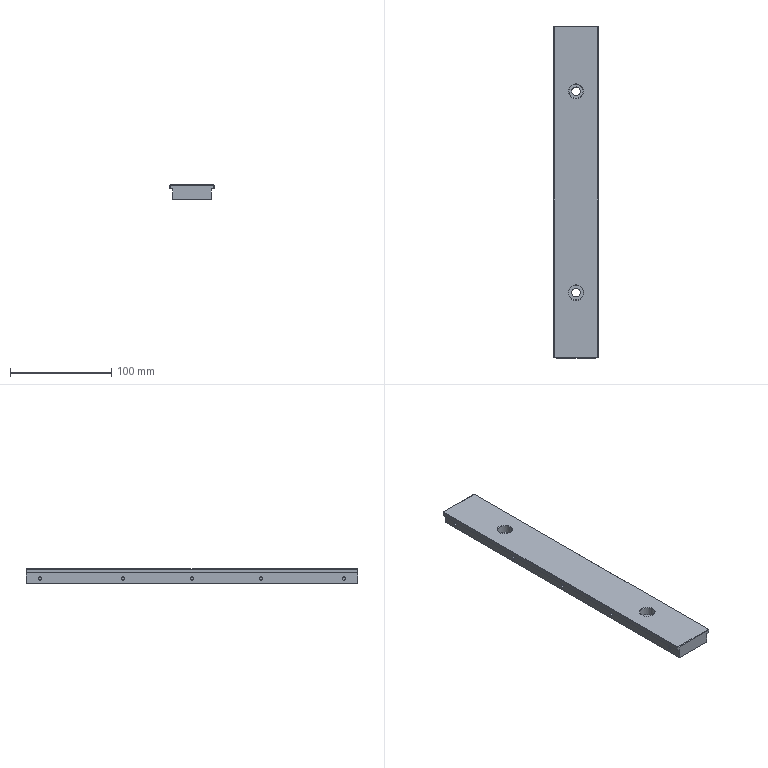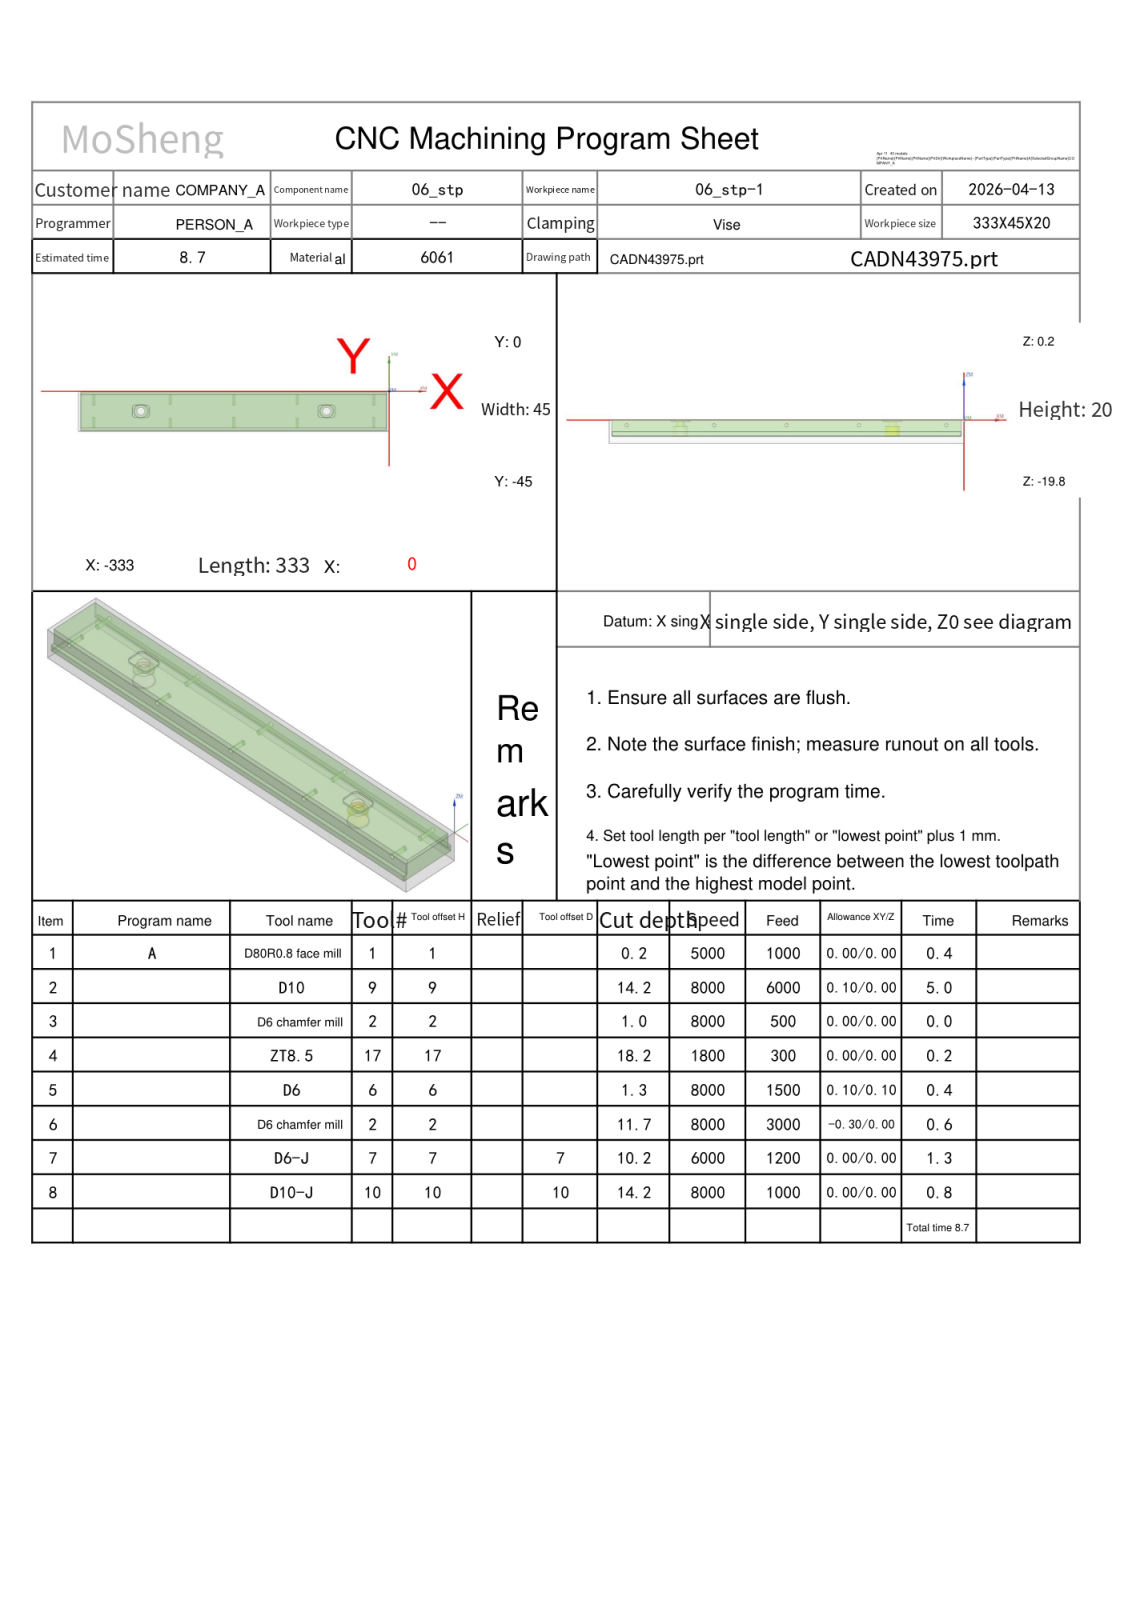NC program | NX | posted by the shop | part box 44 x 328 x 14 mm
Whole program:
%
O0001
(Machine time: 10.41 MIN)
(===Total Tool:7===)
(T1=D80R0.8 face mill D=80.  R=0.8  D-  H01 Z=-0.   )
(T9=D10     D=10.  R=0.   D-  H09 Z=-14.  )
(T2=D6 chamfer mill   D=6.   R=0.   D-  H02 Z=-11.5 )
(T17=ZT8.5  D=8.5  DR_a=118 D-  H17 Z=-18.  )
(T6=D6      D=6.   R=0.   D-  H06 Z=-1.1  )
(T7=D6-J    D=6.   R=0.   D7  H07 Z=-10.  )
(T10=D10-J  D=10.  R=0.   D10 H10 Z=-14.  )
G80 G90 G17 G49 G40
G91 G28 Z0
M01
N1 T01 M06
(D80R0.8 face mill  D=80. R=0.8 H=01 ce=0.00 di=0.00)
G00 G90 G54 X-375.5 Y-22.5 M03 S5000
G43 H01 Z20.
M08
Z2.
G01 Z0.0 F1000.
X-370.5
X37.5
X42.5
Z2.
G00 Z20.
G91 G28 Z0.0
M05
M09
G91 G28 Z0.0
M01
N2 T09 M06
(D10  D=10. R=0. H=09 ce=0.10 di=0.00)
G00 G90 G54 X-166.5 Y4.6 M03 S8000
G43 H09 Z20.
M08
Z.5
G01 X-3. Z.339 F5000.
G02 X.606 Y3.106 Z.335 I0.0 J-5.1
G01 X1.106 Y2.606 Z.334
G02 X2.6 Y-1. Z.33 I-3.606 J-3.606
G01 Y-44. Z.288
G02 X1.106 Y-47.606 Z.284 I-5.1 J0.0
G01 X.606 Y-48.106 Z.283
G02 X-3. Y-49.6 Z.279 I-3.606 J3.606
G01 X-330. Z-.043
G02 X-333.606 Y-48.106 Z-.047 I0.0 J5.1
G01 X-334.106 Y-47.606
G02 X-335.6 Y-44. Z-.051 I3.606 J3.606
G01 Y-1. Z-.094
G02 X-334.106 Y2.606 Z-.097 I5.1 J0.0
G01 X-333.606 Y3.106 Z-.098
G02 X-330. Y4.6 Z-.102 I3.606 J-3.606
G01 X-3. Z-.424
G02 X.606 Y3.106 Z-.428 I0.0 J-5.1
G01 X1.106 Y2.606 Z-.429
G02 X2.6 Y-1. Z-.433 I-3.606 J-3.606
G01 Y-44. Z-.475
G02 X1.106 Y-47.606 Z-.479 I-5.1 J0.0
G01 X.606 Y-48.106 Z-.48
G02 X-3. Y-49.6 Z-.484 I-3.606 J3.606
G01 X-330. Z-.806
G02 X-333.606 Y-48.106 Z-.81 I0.0 J5.1
G01 X-334.106 Y-47.606
G02 X-335.6 Y-44. Z-.814 I3.606 J3.606
G01 Y-1. Z-.857
G02 X-334.106 Y2.606 Z-.861 I5.1 J0.0
G01 X-333.606 Y3.106
G02 X-330. Y4.6 Z-.865 I3.606 J-3.606
G01 X-3. Z-1.187
G02 X.606 Y3.106 Z-1.191 I0.0 J-5.1
G01 X1.106 Y2.606 Z-1.192
G02 X2.6 Y-1. Z-1.196 I-3.606 J-3.606
G01 Y-44. Z-1.238
G02 X1.106 Y-47.606 Z-1.242 I-5.1 J0.0
G01 X.606 Y-48.106 Z-1.243
G02 X-3. Y-49.6 Z-1.247 I-3.606 J3.606
G01 X-330. Z-1.569
G02 X-333.606 Y-48.106 Z-1.573 I0.0 J5.1
G01 X-334.106 Y-47.606 Z-1.574
G02 X-335.6 Y-44. Z-1.578 I3.606 J3.606
G01 Y-1. Z-1.62
G02 X-334.106 Y2.606 Z-1.624 I5.1 J0.0
G01 X-333.606 Y3.106 Z-1.625
G02 X-330. Y4.6 Z-1.628 I3.606 J-3.606
G01 X-3. Z-1.951
G02 X.606 Y3.106 Z-1.954 I0.0 J-5.1
G01 X1.106 Y2.606 Z-1.955
G02 X2.6 Y-1. Z-1.959 I-3.606 J-3.606
G01 Y-44. Z-2.001
G02 X1.106 Y-47.606 Z-2.005 I-5.1 J0.0
G01 X.606 Y-48.106 Z-2.006
G02 X-3. Y-49.6 Z-2.01 I-3.606 J3.606
G01 X-330. Z-2.332
G02 X-333.606 Y-48.106 Z-2.336 I0.0 J5.1
G01 X-334.106 Y-47.606 Z-2.337
G02 X-335.6 Y-44. Z-2.341 I3.606 J3.606
G01 Y-1. Z-2.383
G02 X-334.106 Y2.606 Z-2.387 I5.1 J0.0
G01 X-333.606 Y3.106 Z-2.388
G02 X-330. Y4.6 Z-2.392 I3.606 J-3.606
G01 X-3. Z-2.714
G02 X.606 Y3.106 Z-2.718 I0.0 J-5.1
G01 X1.106 Y2.606
G02 X2.6 Y-1. Z-2.722 I-3.606 J-3.606
G01 Y-44. Z-2.765
G02 X1.106 Y-47.606 Z-2.769 I-5.1 J0.0
G01 X.606 Y-48.106
G02 X-3. Y-49.6 Z-2.773 I-3.606 J3.606
G01 X-330. Z-3.095
G02 X-333.606 Y-48.106 Z-3.099 I0.0 J5.1
G01 X-334.106 Y-47.606 Z-3.1
G02 X-335.6 Y-44. Z-3.104 I3.606 J3.606
G01 Y-1. Z-3.146
G02 X-334.106 Y2.606 Z-3.15 I5.1 J0.0
G01 X-333.606 Y3.106 Z-3.151
G02 X-330. Y4.6 Z-3.155 I3.606 J-3.606
G01 X-3. Z-3.477
G02 X.606 Y3.106 Z-3.481 I0.0 J-5.1
G01 X1.106 Y2.606
G02 X2.6 Y-1. Z-3.485 I-3.606 J-3.606
G01 Y-44. Z-3.528
G02 X1.106 Y-47.606 Z-3.532 I-5.1 J0.0
G01 X.606 Y-48.106
G02 X-3. Y-49.6 Z-3.536 I-3.606 J3.606
G01 X-330. Z-3.858
G02 X-333.606 Y-48.106 Z-3.862 I0.0 J5.1
G01 X-334.106 Y-47.606 Z-3.863
G02 X-335.6 Y-44. Z-3.867 I3.606 J3.606
G01 Y-1. Z-3.909
G02 X-334.106 Y2.606 Z-3.913 I5.1 J0.0
G01 X-333.606 Y3.106 Z-3.914
G02 X-330. Y4.6 Z-3.918 I3.606 J-3.606
G01 X-3. Z-4.24
G02 X.606 Y3.106 Z-4.244 I0.0 J-5.1
G01 X1.106 Y2.606 Z-4.245
G02 X2.6 Y-1. Z-4.249 I-3.606 J-3.606
G01 Y-44. Z-4.291
G02 X1.106 Y-47.606 Z-4.295 I-5.1 J0.0
G01 X.606 Y-48.106 Z-4.296
G02 X-3. Y-49.6 Z-4.299 I-3.606 J3.606
G01 X-330. Z-4.622
G02 X-333.606 Y-48.106 Z-4.626 I0.0 J5.1
G01 X-334.106 Y-47.606
G02 X-335.6 Y-44. Z-4.63 I3.606 J3.606
G01 Y-1. Z-4.672
G02 X-334.106 Y2.606 Z-4.676 I5.1 J0.0
G01 X-333.606 Y3.106 Z-4.677
G02 X-330. Y4.6 Z-4.681 I3.606 J-3.606
G01 X-3. Z-5.003
G02 X.606 Y3.106 Z-5.007 I0.0 J-5.1
G01 X1.106 Y2.606 Z-5.008
G02 X2.6 Y-1. Z-5.012 I-3.606 J-3.606
G01 Y-44. Z-5.054
G02 X1.106 Y-47.606 Z-5.058 I-5.1 J0.0
G01 X.606 Y-48.106 Z-5.059
G02 X-3. Y-49.6 Z-5.063 I-3.606 J3.606
G01 X-330. Z-5.385
G02 X-333.606 Y-48.106 Z-5.389 I0.0 J5.1
G01 X-334.106 Y-47.606
G02 X-335.6 Y-44. Z-5.393 I3.606 J3.606
G01 Y-1. Z-5.436
G02 X-334.106 Y2.606 Z-5.44 I5.1 J0.0
G01 X-333.606 Y3.106
G02 X-330. Y4.6 Z-5.444 I3.606 J-3.606
G01 X-3. Z-5.766
G02 X.606 Y3.106 Z-5.77 I0.0 J-5.1
G01 X1.106 Y2.606 Z-5.771
G02 X2.6 Y-1. Z-5.775 I-3.606 J-3.606
G01 Y-44. Z-5.817
G02 X1.106 Y-47.606 Z-5.821 I-5.1 J0.0
G01 X.606 Y-48.106 Z-5.822
G02 X-3. Y-49.6 Z-5.826 I-3.606 J3.606
G01 X-330. Z-6.148
G02 X-333.606 Y-48.106 Z-6.152 I0.0 J5.1
G01 X-334.106 Y-47.606 Z-6.153
G02 X-335.6 Y-44. Z-6.156 I3.606 J3.606
G01 Y-1. Z-6.199
G02 X-334.106 Y2.606 Z-6.203 I5.1 J0.0
G01 X-333.606 Y3.106
G02 X-330. Y4.6 Z-6.207 I3.606 J-3.606
G01 X-3. Z-6.529
G02 X.606 Y3.106 Z-6.533 I0.0 J-5.1
G01 X1.106 Y2.606 Z-6.534
G02 X2.6 Y-1. Z-6.538 I-3.606 J-3.606
G01 Y-44. Z-6.58
G02 X1.106 Y-47.606 Z-6.584 I-5.1 J0.0
G01 X.606 Y-48.106 Z-6.585
G02 X-3. Y-49.6 Z-6.589 I-3.606 J3.606
G01 X-330. Z-6.911
G02 X-333.606 Y-48.106 Z-6.915 I0.0 J5.1
G01 X-334.106 Y-47.606 Z-6.916
G02 X-335.6 Y-44. Z-6.92 I3.606 J3.606
G01 Y-1. Z-6.962
G02 X-334.106 Y2.606 Z-6.966 I5.1 J0.0
G01 X-333.606 Y3.106 Z-6.967
G02 X-330. Y4.6 Z-6.971 I3.606 J-3.606
G01 X-3. Z-7.293
G02 X.606 Y3.106 Z-7.297 I0.0 J-5.1
G01 X1.106 Y2.606
G02 X2.6 Y-1. Z-7.301 I-3.606 J-3.606
G01 Y-44. Z-7.344
G02 X1.106 Y-47.606 Z-7.347 I-5.1 J0.0
G01 X.606 Y-48.106 Z-7.348
G02 X-3. Y-49.6 Z-7.352 I-3.606 J3.606
G01 X-330. Z-7.674
G02 X-333.606 Y-48.106 Z-7.678 I0.0 J5.1
G01 X-334.106 Y-47.606 Z-7.679
G02 X-335.6 Y-44. Z-7.683 I3.606 J3.606
G01 Y-1. Z-7.725
G02 X-334.106 Y2.606 Z-7.729 I5.1 J0.0
G01 X-333.606 Y3.106 Z-7.73
G02 X-330. Y4.6 Z-7.734 I3.606 J-3.606
G01 X-3. Z-8.056
G02 X.606 Y3.106 Z-8.06 I0.0 J-5.1
G01 X1.106 Y2.606
G02 X2.6 Y-1. Z-8.064 I-3.606 J-3.606
G01 Y-44. Z-8.107
G02 X1.106 Y-47.606 Z-8.111 I-5.1 J0.0
G01 X.606 Y-48.106
G02 X-3. Y-49.6 Z-8.115 I-3.606 J3.606
G01 X-330. Z-8.437
G02 X-333.606 Y-48.106 Z-8.441 I0.0 J5.1
G01 X-334.106 Y-47.606 Z-8.442
G02 X-335.6 Y-44. Z-8.446 I3.606 J3.606
G01 Y-1. Z-8.488
G02 X-334.106 Y2.606 Z-8.492 I5.1 J0.0
G01 X-333.606 Y3.106 Z-8.493
G02 X-330. Y4.6 Z-8.497 I3.606 J-3.606
G01 X-3. Z-8.819
G02 X.606 Y3.106 Z-8.823 I0.0 J-5.1
G01 X1.106 Y2.606 Z-8.824
G02 X2.6 Y-1. Z-8.828 I-3.606 J-3.606
G01 Y-44. Z-8.87
G02 X1.106 Y-47.606 Z-8.874 I-5.1 J0.0
G01 X.606 Y-48.106 Z-8.875
G02 X-3. Y-49.6 Z-8.878 I-3.606 J3.606
G01 X-330. Z-9.201
G02 X-333.606 Y-48.106 Z-9.204 I0.0 J5.1
G01 X-334.106 Y-47.606 Z-9.205
G02 X-335.6 Y-44. Z-9.209 I3.606 J3.606
G01 Y-1. Z-9.251
G02 X-334.106 Y2.606 Z-9.255 I5.1 J0.0
G01 X-333.606 Y3.106 Z-9.256
G02 X-330. Y4.6 Z-9.26 I3.606 J-3.606
G01 X-3. Z-9.582
G02 X.606 Y3.106 Z-9.586 I0.0 J-5.1
G01 X1.106 Y2.606 Z-9.587
G02 X2.6 Y-1. Z-9.591 I-3.606 J-3.606
G01 Y-44. Z-9.633
G02 X1.106 Y-47.606 Z-9.637 I-5.1 J0.0
G01 X.606 Y-48.106 Z-9.638
G02 X-3. Y-49.6 Z-9.642 I-3.606 J3.606
G01 X-330. Z-9.964
G02 X-333.606 Y-48.106 Z-9.968 I0.0 J5.1
G01 X-334.106 Y-47.606
G02 X-335.6 Y-44. Z-9.972 I3.606 J3.606
G01 Y-1. Z-10.015
G02 X-334.106 Y2.606 Z-10.019 I5.1 J0.0
G01 X-333.606 Y3.106
G02 X-330. Y4.6 Z-10.023 I3.606 J-3.606
G01 X-3. Z-10.345
G02 X.606 Y3.106 Z-10.349 I0.0 J-5.1
G01 X1.106 Y2.606 Z-10.35
G02 X2.6 Y-1. Z-10.354 I-3.606 J-3.606
G01 Y-44. Z-10.396
G02 X1.106 Y-47.606 Z-10.4 I-5.1 J0.0
G01 X.606 Y-48.106 Z-10.401
G02 X-3. Y-49.6 Z-10.405 I-3.606 J3.606
G01 X-330. Z-10.727
G02 X-333.606 Y-48.106 Z-10.731 I0.0 J5.1
G01 X-334.106 Y-47.606
G02 X-335.6 Y-44. Z-10.735 I3.606 J3.606
G01 Y-1. Z-10.778
G02 X-334.106 Y2.606 Z-10.782 I5.1 J0.0
G01 X-333.606 Y3.106
G02 X-330. Y4.6 Z-10.786 I3.606 J-3.606
G01 X-3. Z-11.108
G02 X.606 Y3.106 Z-11.112 I0.0 J-5.1
G01 X1.106 Y2.606 Z-11.113
G02 X2.6 Y-1. Z-11.117 I-3.606 J-3.606
G01 Y-44. Z-11.159
G02 X1.106 Y-47.606 Z-11.163 I-5.1 J0.0
G01 X.606 Y-48.106 Z-11.164
G02 X-3. Y-49.6 Z-11.168 I-3.606 J3.606
G01 X-330. Z-11.49
G02 X-333.606 Y-48.106 Z-11.494 I0.0 J5.1
G01 X-334.106 Y-47.606 Z-11.495
G02 X-335.6 Y-44. Z-11.499 I3.606 J3.606
G01 Y-1. Z-11.541
G02 X-334.106 Y2.606 Z-11.545 I5.1 J0.0
G01 X-333.606 Y3.106 Z-11.546
G02 X-330. Y4.6 Z-11.549 I3.606 J-3.606
G01 X-3. Z-11.872
G02 X.606 Y3.106 Z-11.876 I0.0 J-5.1
G01 X1.106 Y2.606
G02 X2.6 Y-1. Z-11.88 I-3.606 J-3.606
G01 Y-44. Z-11.922
G02 X1.106 Y-47.606 Z-11.926 I-5.1 J0.0
G01 X.606 Y-48.106 Z-11.927
G02 X-3. Y-49.6 Z-11.931 I-3.606 J3.606
G01 X-330. Z-12.253
G02 X-333.606 Y-48.106 Z-12.257 I0.0 J5.1
G01 X-334.106 Y-47.606 Z-12.258
G02 X-335.6 Y-44. Z-12.262 I3.606 J3.606
G01 Y-1. Z-12.304
G02 X-334.106 Y2.606 Z-12.308 I5.1 J0.0
G01 X-333.606 Y3.106 Z-12.309
G02 X-330. Y4.6 Z-12.313 I3.606 J-3.606
G01 X-3. Z-12.635
G02 X.606 Y3.106 Z-12.639 I0.0 J-5.1
G01 X1.106 Y2.606
G02 X2.6 Y-1. Z-12.643 I-3.606 J-3.606
G01 Y-44. Z-12.686
G02 X1.106 Y-47.606 Z-12.69 I-5.1 J0.0
G01 X.606 Y-48.106
G02 X-3. Y-49.6 Z-12.694 I-3.606 J3.606
G01 X-330. Z-13.016
G02 X-333.606 Y-48.106 Z-13.02 I0.0 J5.1
G01 X-334.106 Y-47.606 Z-13.021
G02 X-335.6 Y-44. Z-13.025 I3.606 J3.606
G01 Y-1. Z-13.067
G02 X-334.106 Y2.606 Z-13.071 I5.1 J0.0
G01 X-333.606 Y3.106 Z-13.072
G02 X-330. Y4.6 Z-13.076 I3.606 J-3.606
G01 X-3. Z-13.398
G02 X.606 Y3.106 Z-13.402 I0.0 J-5.1
G01 X1.106 Y2.606 Z-13.403
G02 X2.6 Y-1. Z-13.406 I-3.606 J-3.606
G01 Y-44. Z-13.449
G02 X1.106 Y-47.606 Z-13.453 I-5.1 J0.0
G01 X.606 Y-48.106
G02 X-3. Y-49.6 Z-13.457 I-3.606 J3.606
G01 X-330. Z-13.779
G02 X-333.606 Y-48.106 Z-13.783 I0.0 J5.1
G01 X-334.106 Y-47.606 Z-13.784
G02 X-335.6 Y-44. Z-13.788 I3.606 J3.606
G01 Y-1. Z-13.83
G02 X-334.106 Y2.606 Z-13.834 I5.1 J0.0
G01 X-333.606 Y3.106 Z-13.835
G02 X-330. Y4.6 Z-13.839 I3.606 J-3.606
G01 X-166.5 Z-14.
X-3.
G02 X.606 Y3.106 I0.0 J-5.1
G01 X1.106 Y2.606
G02 X2.6 Y-1. I-3.606 J-3.606
G01 Y-44.
G02 X1.106 Y-47.606 I-5.1 J0.0
G01 X.606 Y-48.106
G02 X-3. Y-49.6 I-3.606 J3.606
G01 X-330.
G02 X-333.606 Y-48.106 I0.0 J5.1
G01 X-334.106 Y-47.606
G02 X-335.6 Y-44. I3.606 J3.606
G01 Y-1.
G02 X-334.106 Y2.606 I5.1 J0.0
G01 X-333.606 Y3.106
G02 X-330. Y4.6 I3.606 J-3.606
G01 X-166.5
X-166.
Z-13.
G00 Z20.
G00 G90 X6.218 Y-46.55 M03 S8000
Z20.
Z-.588
G01 X-2.5 F6000.
X-330.5
X-339.218
G00 Z-1.176
G01 X-330.5
X-2.5
X6.218
G00 Z-1.765
G01 X-2.5
X-330.5
X-339.218
G00 Z-2.353
G01 X-330.5
X-2.5
X6.218
G00 Z-2.941
G01 X-2.5
X-330.5
X-339.218
G00 Z-3.529
G01 X-330.5
X-2.5
X6.218
G00 Z-4.118
G01 X-2.5
X-330.5
X-339.218
G00 Z-4.706
G01 X-330.5
X-2.5
X6.218
G00 Z-5.294
G01 X-2.5
X-330.5
X-339.218
G00 Z-5.882
G01 X-330.5
X-2.5
X6.218
G00 Z-6.471
G01 X-2.5
X-330.5
X-339.218
G00 Z-7.059
G01 X-330.5
X-2.5
X6.218
G00 Z-7.647
G01 X-2.5
X-330.5
X-339.218
G00 Z-8.235
G01 X-330.5
X-2.5
X6.218
G00 Z-8.824
G01 X-2.5
X-330.5
X-339.218
G00 Z-9.412
G01 X-330.5
X-2.5
X6.218
G00 Z20.
X-339.218 Y1.55
Z-.588
G01 X-330.5
X-2.5
X6.218
G00 Z-1.176
G01 X-2.5
X-330.5
X-339.218
G00 Z-1.765
G01 X-330.5
X-2.5
X6.218
G00 Z-2.353
G01 X-2.5
X-330.5
X-339.218
G00 Z-2.941
G01 X-330.5
X-2.5
X6.218
G00 Z-3.529
G01 X-2.5
X-330.5
X-339.218
G00 Z-4.118
G01 X-330.5
X-2.5
X6.218
G00 Z-4.706
G01 X-2.5
X-330.5
X-339.218
G00 Z-5.294
G01 X-330.5
X-2.5
X6.218
G00 Z-5.882
G01 X-2.5
X-330.5
X-339.218
G00 Z-6.471
G01 X-330.5
X-2.5
X6.218
G00 Z-7.059
G01 X-2.5
X-330.5
X-339.218
G00 Z-7.647
G01 X-330.5
X-2.5
X6.218
G00 Z-8.235
G01 X-2.5
X-330.5
X-339.218
G00 Z-8.824
G01 X-330.5
X-2.5
X6.218
G00 Z-9.412
G01 X-2.5
X-330.5
X-339.218
G00 Z20.
G91 G28 Z0.0
M05
M09
G91 G28 Z0.0
M01
N3 T02 M06
(D6 chamfer mill  D=6. R=0. H=02 ce=0.00 di=0.10)
G00 G90 G54 X-67. Y-22.5 M03 S8000
G43 H02 Z20.
M08
G98 G81 X-67. Y-22.5 Z-.8 R1. F500.
X-266.
G80
G00 Z20.
G91 G28 Z0.0
M05
M09
G91 G28 Z0.0
M01
N4 T17 M06
(ZT8.5 D=8.5 DR_a=118 H=17)
G00 G90 G54 X-67. Y-22.5 M03 S1800
G43 H17 Z20.
M08
G98 G83 X-67. Y-22.5 Z-18. R1. F300. Q3.
X-266.
G80
G00 Z20.
G91 G28 Z0.0
M05
M09
G91 G28 Z0.0
M01
N5 T06 M06
(D6  D=6. R=0. H=06 ce=0.10 di=0.10)
G00 G90 G54 X-62.018 Y-18.5 M03 S8000
G43 H06 Z20.
M08
Z1.
G01 X-72.8 Z.435 F1500.
X-72.914 Z.429
X-73. Y-18.586 Z.423
Y-26.414 Z.012
X-72.914 Y-26.5 Z.006
X-72.8 Z0.0
X-61.2 Z-.054
G03 X-61. Y-26.3 Z-.055 I0.0 J.2
G01 Y-18.7 Z-.09
G03 X-61.2 Y-18.5 Z-.092 I-.2 J0.0
G01 X-72.8 Z-.145
G03 X-73. Y-18.7 Z-.147 I0.0 J-.2
G01 Y-26.3 Z-.182
G03 X-72.8 Y-26.5 Z-.183 I.2 J0.0
G01 X-61.2 Z-.237
G03 X-61. Y-26.3 Z-.238 I0.0 J.2
G01 Y-18.7 Z-.274
G03 X-61.2 Y-18.5 Z-.275 I-.2 J0.0
G01 X-72.8 Z-.329
G03 X-73. Y-18.7 Z-.33 I0.0 J-.2
G01 Y-26.3 Z-.365
G03 X-72.8 Y-26.5 Z-.367 I.2 J0.0
G01 X-61.2 Z-.42
G03 X-61. Y-26.3 Z-.422 I0.0 J.2
G01 Y-18.7 Z-.457
G03 X-61.2 Y-18.5 Z-.458 I-.2 J0.0
G01 X-72.8 Z-.512
G03 X-73. Y-18.7 Z-.513 I0.0 J-.2
G01 Y-26.3 Z-.549
G03 X-72.8 Y-26.5 Z-.55 I.2 J0.0
G01 X-61.2 Z-.604
G03 X-61. Y-26.3 Z-.605 I0.0 J.2
G01 Y-18.7 Z-.64
G03 X-61.2 Y-18.5 Z-.642 I-.2 J0.0
G01 X-72.8 Z-.695
G03 X-73. Y-18.7 Z-.697 I0.0 J-.2
G01 Y-26.3 Z-.732
G03 X-72.8 Y-26.5 Z-.733 I.2 J0.0
G01 X-61.2 Z-.787
G03 X-61. Y-26.3 Z-.788 I0.0 J.2
G01 Y-18.7 Z-.824
G03 X-61.2 Y-18.5 Z-.825 I-.2 J0.0
G01 X-72.8 Z-.879
G03 X-73. Y-18.7 Z-.88 I0.0 J-.2
G01 Y-26.3 Z-.915
G03 X-72.8 Y-26.5 Z-.917 I.2 J0.0
G01 X-61.2 Z-.97
G03 X-61. Y-26.3 Z-.972 I0.0 J.2
G01 Y-18.7 Z-1.007
G03 X-61.2 Y-18.5 Z-1.008 I-.2 J0.0
G01 X-72.8 Z-1.062
G03 X-73. Y-18.7 Z-1.063 I0.0 J-.2
G01 Y-26.3 Z-1.099
G03 X-72.8 Y-26.5 Z-1.1 I.2 J0.0
G01 X-61.2
G03 X-61. Y-26.3 I0.0 J.2
G01 Y-18.7
G03 X-61.2 Y-18.5 I-.2 J0.0
G01 X-72.8
G03 X-73. Y-18.7 I0.0 J-.2
G01 Y-26.3
G03 X-72.8 Y-26.5 I.2 J0.0
G01 X-72.4
Z-.1
G00 Z20.
X-261.018 Y-18.5
Z1.
G01 X-271.8 Z.435
X-271.914 Z.429
X-272. Y-18.586 Z.423
Y-26.414 Z.012
X-271.914 Y-26.5 Z.006
X-271.8 Z0.0
X-260.2 Z-.054
G03 X-260. Y-26.3 Z-.055 I0.0 J.2
G01 Y-18.7 Z-.09
G03 X-260.2 Y-18.5 Z-.092 I-.2 J0.0
G01 X-271.8 Z-.145
G03 X-272. Y-18.7 Z-.147 I0.0 J-.2
G01 Y-26.3 Z-.182
G03 X-271.8 Y-26.5 Z-.183 I.2 J0.0
G01 X-260.2 Z-.237
G03 X-260. Y-26.3 Z-.238 I0.0 J.2
G01 Y-18.7 Z-.274
G03 X-260.2 Y-18.5 Z-.275 I-.2 J0.0
G01 X-271.8 Z-.329
G03 X-272. Y-18.7 Z-.33 I0.0 J-.2
G01 Y-26.3 Z-.365
G03 X-271.8 Y-26.5 Z-.367 I.2 J0.0
G01 X-260.2 Z-.42
G03 X-260. Y-26.3 Z-.422 I0.0 J.2
G01 Y-18.7 Z-.457
G03 X-260.2 Y-18.5 Z-.458 I-.2 J0.0
G01 X-271.8 Z-.512
G03 X-272. Y-18.7 Z-.513 I0.0 J-.2
G01 Y-26.3 Z-.549
G03 X-271.8 Y-26.5 Z-.55 I.2 J0.0
G01 X-260.2 Z-.604
G03 X-260. Y-26.3 Z-.605 I0.0 J.2
G01 Y-18.7 Z-.64
G03 X-260.2 Y-18.5 Z-.642 I-.2 J0.0
G01 X-271.8 Z-.695
G03 X-272. Y-18.7 Z-.697 I0.0 J-.2
G01 Y-26.3 Z-.732
G03 X-271.8 Y-26.5 Z-.733 I.2 J0.0
G01 X-260.2 Z-.787
G03 X-260. Y-26.3 Z-.788 I0.0 J.2
G01 Y-18.7 Z-.824
G03 X-260.2 Y-18.5 Z-.825 I-.2 J0.0
G01 X-271.8 Z-.879
G03 X-272. Y-18.7 Z-.88 I0.0 J-.2
G01 Y-26.3 Z-.915
G03 X-271.8 Y-26.5 Z-.917 I.2 J0.0
G01 X-260.2 Z-.97
G03 X-260. Y-26.3 Z-.972 I0.0 J.2
G01 Y-18.7 Z-1.007
G03 X-260.2 Y-18.5 Z-1.008 I-.2 J0.0
G01 X-271.8 Z-1.062
G03 X-272. Y-18.7 Z-1.063 I0.0 J-.2
G01 Y-26.3 Z-1.099
G03 X-271.8 Y-26.5 Z-1.1 I.2 J0.0
G01 X-260.2
G03 X-260. Y-26.3 I0.0 J.2
G01 Y-18.7
G03 X-260.2 Y-18.5 I-.2 J0.0
G01 X-271.8
G03 X-272. Y-18.7 I0.0 J-.2
G01 Y-26.3
G03 X-271.8 Y-26.5 I.2 J0.0
G01 X-271.4
Z-.1
G00 Z20.
G91 G28 Z0.0
M05
M09
G91 G28 Z0.0
M01
N6 T02 M06
(D6 chamfer mill  D=6. R=0. H=02 ce=0.00 di=0.00)
G00 G90 G54 X-166.25 Y-43.578 M03 S8000
G43 H02 Z20.
M08
Z2.099
G01 Z-1.5 F3000.
G03 X-166.17 Y-43.278 I-.52 J.3
X-166.47 Y-42.758 I-.6 J0.0
G01 X-166.5 Y-42.75
X-330.5
G02 X-331.8 Y-41.45 I0.0 J1.3
G01 Y-3.55
G02 X-330.5 Y-2.25 I1.3 J0.0
G01 X-2.5
G02 X-1.2 Y-3.55 I0.0 J-1.3
G01 Y-41.45
G02 X-2.5 Y-42.75 I-1.3 J0.0
G01 X-166.5
X-166.53 Y-42.758
G03 X-166.83 Y-43.278 I.3 J-.52
X-166.75 Y-43.578 I.6 J0.0
G01 Z2.099
G00 Z20.
X-332.278 Y.177
Z1.755
G01 Z-11.5
G03 X-331.716 Y-.211 I.562 J.211
X-331.505 Y-.173 I0.0 J.6
G01 X-331.48 Y-.155
X-331.419 Y-.081
X-330.919 Y.419
X-330.722 Y.581
X-330.497 Y.701
X-330.254 Y.775
X-330. Y.8
X-328.723
X-327.445
X-324.891
X-321.059
X-319.781
X-315.949
X-313.395
X-312.117
X-309.563
X-305.73
X-303.176
X-301.898
X-298.066
X-296.789
X-294.234
X-290.402
X-289.125
X-285.293
X-282.738
X-281.461
X-277.629
X-276.352
X-273.797
X-269.965
X-267.41
X-266.133
X-263.578
X-259.746
X-258.469
X-254.637
X-252.082
X-250.805
X-248.25
X-244.418
X-241.863
X-240.586
X-236.754
X-235.477
X-232.922
X-229.09
X-226.535
X-225.258
X-222.703
X-218.871
X-217.594
X-213.762
X-211.207
X-209.93
X-206.098
X-204.82
X-202.266
X-198.434
X-197.156
X-193.324
X-190.77
X-189.492
X-186.938
X-183.105
X-180.551
X-179.273
X-175.441
X-174.164
X-171.609
X-166.5
X-162.668
X-160.113
X-158.836
X-155.004
X-153.727
X-151.172
X-147.34
X-144.785
X-143.508
X-140.953
X-137.121
X-135.844
X-132.012
X-129.457
X-128.18
X-124.348
X-123.07
X-120.516
X-116.684
X-115.406
X-111.574
X-109.02
X-107.742
X-105.188
X-101.355
X-98.801
X-97.523
X-93.691
X-92.414
X-89.859
X-86.027
X-83.473
X-82.195
X-79.641
X-75.809
X-74.531
X-70.699
X-68.145
X-66.867
X-64.313
X-60.48
X-57.926
X-56.648
X-52.816
X-51.539
X-48.984
X-45.152
X-43.875
X-40.043
X-37.488
X-36.211
X-32.379
X-31.102
X-28.547
X-24.715
X-22.16
X-20.883
X-18.328
X-14.496
X-13.219
X-9.387
X-6.832
X-5.555
X-3.
X-2.746 Y.775
X-2.503 Y.701
X-2.278 Y.581
X-2.081 Y.419
X-1.581 Y-.081
X-1.52 Y-.155
X-1.495 Y-.173
G03 X-1.284 Y-.211 I.211 J.562
X-.722 Y.177 I0.0 J.6
G01 Z1.755
G00 Z20.
Y-45.177
Z1.755
G01 Z-11.5
G03 X-1.284 Y-44.789 I-.562 J-.211
X-1.495 Y-44.827 I0.0 J-.6
G01 X-1.52 Y-44.845
X-1.581 Y-44.919
X-2.081 Y-45.419
X-2.278 Y-45.581
X-2.503 Y-45.701
X-2.746 Y-45.775
X-3. Y-45.8
X-4.277
X-5.555
X-8.109
X-11.941
X-13.219
X-17.051
X-19.605
X-20.883
X-23.438
X-27.27
X-29.824
X-31.102
X-34.934
X-36.211
X-38.766
X-42.598
X-43.875
X-47.707
X-50.262
X-51.539
X-55.371
X-56.648
X-59.203
X-63.035
X-65.59
X-66.867
X-69.422
X-73.254
X-74.531
X-78.363
X-80.918
X-82.195
X-84.75
X-88.582
X-91.137
X-92.414
X-96.246
X-97.523
X-100.078
X-103.91
X-106.465
X-107.742
X-110.297
X-114.129
X-115.406
X-119.238
X-121.793
X-123.07
X-126.902
X-128.18
X-130.734
X-134.566
X-135.844
X-139.676
X-142.23
X-143.508
X-146.063
X-149.895
X-152.449
X-153.727
X-157.559
X-158.836
X-161.391
X-166.5
X-170.332
X-172.887
X-174.164
X-177.996
X-179.273
X-181.828
X-185.66
X-188.215
X-189.492
X-192.047
X-195.879
X-197.156
X-200.988
X-203.543
X-204.82
X-208.652
X-209.93
X-212.484
X-216.316
X-217.594
X-221.426
X-223.98
X-225.258
X-227.813
X-231.645
X-234.199
X-235.477
X-239.309
X-240.586
X-243.141
X-246.973
X-249.527
X-250.805
X-253.359
X-257.191
X-258.469
X-262.301
X-264.855
X-266.133
X-268.688
X-272.52
X-275.074
X-276.352
X-280.184
X-281.461
X-284.016
X-287.848
X-289.125
X-292.957
X-295.512
X-296.789
X-300.621
X-301.898
X-304.453
X-308.285
X-310.84
X-312.117
X-314.672
X-318.504
X-319.781
X-323.613
X-326.168
X-327.445
X-330.
X-330.254 Y-45.775
X-330.497 Y-45.701
X-330.722 Y-45.581
X-330.919 Y-45.419
X-331.419 Y-44.919
X-331.48 Y-44.845
X-331.505 Y-44.827
G03 X-331.716 Y-44.789 I-.211 J-.562
X-332.278 Y-45.177 I0.0 J-.6
G01 Z1.755
G00 Z20.
G00 G90 X-64.492 Y-22.04 M03 S8000
Z20.
Z-1.7
G01 Z-2.2 F800.
X-64. Y-21.95
G03 X-67. Y-18.95 I-3. J0.0
X-70.55 Y-22.5 I0.0 J-3.55
X-67. Y-26.05 I3.55 J0.0
X-63.45 Y-22.5 I0.0 J3.55
X-67. Y-18.95 I-3.55 J0.0
X-70. Y-21.95 I0.0 J-3.
G01 X-69.508 Y-22.04
Z-1.7
G00 Z20.
X-263.492
Z-1.7
G01 Z-2.2
X-263. Y-21.95
G03 X-266. Y-18.95 I-3. J0.0
X-269.55 Y-22.5 I0.0 J-3.55
X-266. Y-26.05 I3.55 J0.0
X-262.45 Y-22.5 I0.0 J3.55
X-266. Y-18.95 I-3.55 J0.0
X-269. Y-21.95 I0.0 J-3.
G01 X-268.508 Y-22.04
Z-1.7
G00 Z20.
G91 G28 Z0.0
M05
M09
G91 G28 Z0.0
M01
N7 T07 M06
(D6-J  D=6. R=0. H=07 ce=0.00 di=0.00)
G00 G90 G54 X-334.2 Y.55 M03 S6000
G43 H07 Z20.
M08
Z-4.5
G01 Z-5. F1200.
G41 D07
Y.45
G03 X-333.2 Y-.55 I1. J0.0
G01 X.2
G03 X1.2 Y.45 I0.0 J1.
G01 G40 Y.55
Z-4.5
G00 Z20.
X-334.2
Z-9.5
G01 Z-10.
G41 D07
Y.45
G03 X-333.2 Y-.55 I1. J0.0
G01 X.2
G03 X1.2 Y.45 I0.0 J1.
G01 G40 Y.55
Z-9.5
G00 Z20.
Y-45.55
Z-4.5
G01 Z-5.
G41 D07
Y-45.45
G03 X.2 Y-44.45 I-1. J0.0
G01 X-333.2
G03 X-334.2 Y-45.45 I0.0 J-1.
G01 G40 Y-45.55
Z-4.5
G00 Z20.
X1.2
Z-9.5
G01 Z-10.
G41 D07
Y-45.45
G03 X.2 Y-44.45 I-1. J0.0
G01 X-333.2
G03 X-334.2 Y-45.45 I0.0 J-1.
G01 G40 Y-45.55
Z-9.5
G00 Z20.
G00 G90 X-265. Y-19.5 M03 S6000
Z20.
Z-.7
G01 Z-1.2 F1200.
G41 D07
Y-19.4
G03 X-266. Y-18.4 I-1. J0.0
G01 X-271.8
G03 X-272.1 Y-18.7 I0.0 J-.3
G01 Y-26.3
G03 X-271.8 Y-26.6 I.3 J0.0
G01 X-260.2
G03 X-259.9 Y-26.3 I0.0 J.3
G01 Y-18.7
G03 X-260.2 Y-18.4 I-.3 J0.0
G01 X-266.
X-266.5
G03 X-267.5 Y-19.4 I0.0 J-1.
G01 G40 Y-19.5
Z-.7
G00 Z20.
X-66.
Z-.7
G01 Z-1.2
G41 D07
Y-19.4
G03 X-67. Y-18.4 I-1. J0.0
G01 X-72.8
G03 X-73.1 Y-18.7 I0.0 J-.3
G01 Y-26.3
G03 X-72.8 Y-26.6 I.3 J0.0
G01 X-61.2
G03 X-60.9 Y-26.3 I0.0 J.3
G01 Y-18.7
G03 X-61.2 Y-18.4 I-.3 J0.0
G01 X-67.
X-67.5
G03 X-68.5 Y-19.4 I0.0 J-1.
G01 G40 Y-19.5
Z-.7
G00 Z20.
G91 G28 Z0.0
M05
M09
G91 G28 Z0.0
M01
N8 T10 M06
(D10-J  D=10. R=0. H=10 ce=0.00 di=0.00)
G00 G90 G54 X-331.013 Y5.616 M03 S8000
G43 H10 Z20.
M08
Z-13.5
G01 Z-14. F1000.
G41 D10
X-330.997 Y5.417
G03 X-330. Y4.5 I.997 J.083
G01 X-3.
G02 X.536 Y3.036 I0.0 J-5.
G01 X1.036 Y2.536
G02 X2.5 Y-1. I-3.536 J-3.536
G01 Y-44.
G02 X1.036 Y-47.536 I-5. J0.0
G01 X.536 Y-48.036
G02 X-3. Y-49.5 I-3.536 J3.536
G01 X-330.
G02 X-333.536 Y-48.036 I0.0 J5.
G01 X-334.036 Y-47.536
G02 X-335.5 Y-44. I3.536 J3.536
G01 Y-1.
G02 X-334.036 Y2.536 I5. J0.0
G01 X-333.536 Y3.036
G02 X-330. Y4.5 I3.536 J-3.536
G01 X-329.5
G03 X-328.5 Y5.5 I0.0 J1.
G01 G40 Y5.7
Z-13.5
G00 Z20.
M05
M09
G91 G28 Z0.0
G91 G28 Y0.0
M30
%